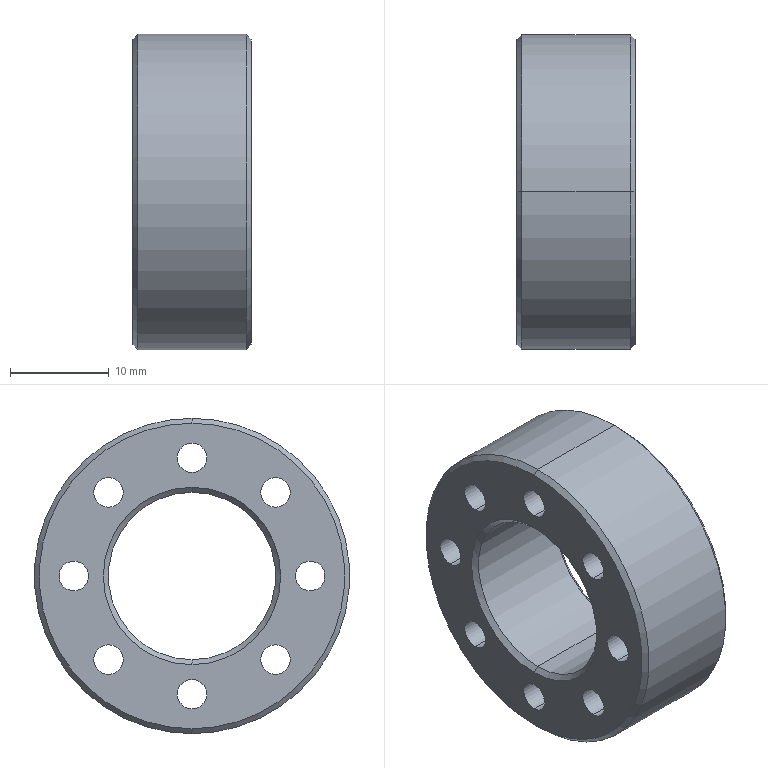Part | STEP file | PN_0034 JIG Block_Default | 1 solid | 30 faces | box 12 x 32 x 32 mm | volume 6210 mm3 | cylinder 20 | cone 8 | plane 2 | commonest cylinder face diameters 3 x16 17 x2 32 x2